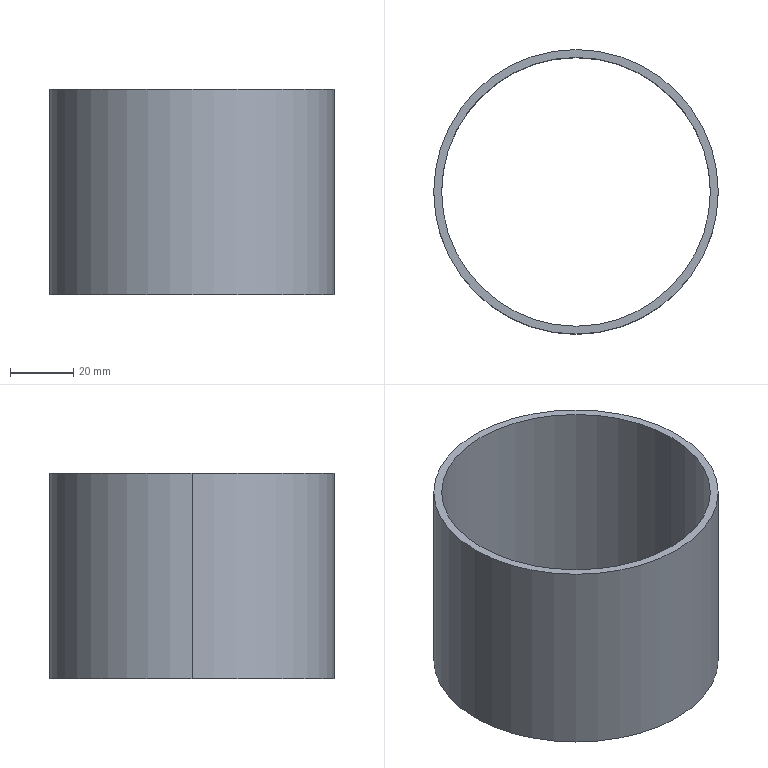Part | SolidWorks | features Extrusion 1 | 1 solid | 6 faces | box 90 x 90 x 65 mm | volume 44670 mm3 | cylinder 4 | plane 2 | commonest cylinder face diameters 85 x2 90 x2
STEP:
#1=CARTESIAN_POINT('',(-42.5,0.,32.5));
#2=VERTEX_POINT('',#1);
#3=CARTESIAN_POINT('',(42.5,0.,32.5));
#4=VERTEX_POINT('',#3);
#5=CARTESIAN_POINT('',(0.,0.,32.5));
#6=DIRECTION('',(0.,0.,1.));
#7=DIRECTION('',(1.,0.,0.));
#8=AXIS2_PLACEMENT_3D('',#5,#6,#7);
#9=CIRCLE('',#8,42.5);
#10=EDGE_CURVE('',#2,#4,#9,.T.);
#11=ORIENTED_EDGE('',*,*,#10,.T.);
#12=CARTESIAN_POINT('',(42.5,0.,-32.5));
#13=VERTEX_POINT('',#12);
#14=CARTESIAN_POINT('',(42.5,0.,32.5));
#15=DIRECTION('',(0.,0.,-1.));
#16=VECTOR('',#15,1000.);
#17=LINE('',#14,#16);
#18=EDGE_CURVE('',#4,#13,#17,.T.);
#19=ORIENTED_EDGE('',*,*,#18,.T.);
#20=CARTESIAN_POINT('',(-42.5,0.,-32.5));
#21=VERTEX_POINT('',#20);
#22=CARTESIAN_POINT('',(0.,0.,-32.5));
#23=DIRECTION('',(0.,0.,1.));
#24=DIRECTION('',(1.,0.,0.));
#25=AXIS2_PLACEMENT_3D('',#22,#23,#24);
#26=CIRCLE('',#25,42.5);
#27=EDGE_CURVE('',#21,#13,#26,.T.);
#28=ORIENTED_EDGE('',*,*,#27,.F.);
#29=CARTESIAN_POINT('',(-42.5,0.,32.5));
#30=DIRECTION('',(0.,0.,-1.));
#31=VECTOR('',#30,1000.);
#32=LINE('',#29,#31);
#33=EDGE_CURVE('',#2,#21,#32,.T.);
#34=ORIENTED_EDGE('',*,*,#33,.F.);
#35=EDGE_LOOP('',(#11,#19,#28,#34));
#36=FACE_OUTER_BOUND('',#35,.T.);
#37=CARTESIAN_POINT('',(0.,0.,32.5));
#38=DIRECTION('',(0.,0.,-1.));
#39=DIRECTION('',(-1.,0.,0.));
#40=AXIS2_PLACEMENT_3D('',#37,#38,#39);
#41=CYLINDRICAL_SURFACE('',#40,42.5);
#42=ADVANCED_FACE('',(#36),#41,.F.);
#43=CARTESIAN_POINT('',(45.,0.,32.5));
#44=VERTEX_POINT('',#43);
#45=CARTESIAN_POINT('',(-45.,0.,32.5));
#46=VERTEX_POINT('',#45);
#47=CARTESIAN_POINT('',(0.,0.,32.5));
#48=DIRECTION('',(0.,0.,1.));
#49=DIRECTION('',(1.,0.,0.));
#50=AXIS2_PLACEMENT_3D('',#47,#48,#49);
#51=CIRCLE('',#50,45.);
#52=EDGE_CURVE('',#44,#46,#51,.T.);
#53=ORIENTED_EDGE('',*,*,#52,.F.);
#54=CARTESIAN_POINT('',(45.,0.,-32.5));
#55=VERTEX_POINT('',#54);
#56=CARTESIAN_POINT('',(45.,0.,32.5));
#57=DIRECTION('',(0.,0.,-1.));
#58=VECTOR('',#57,1000.);
#59=LINE('',#56,#58);
#60=EDGE_CURVE('',#44,#55,#59,.T.);
#61=ORIENTED_EDGE('',*,*,#60,.T.);
#62=CARTESIAN_POINT('',(-45.,0.,-32.5));
#63=VERTEX_POINT('',#62);
#64=CARTESIAN_POINT('',(0.,0.,-32.5));
#65=DIRECTION('',(0.,0.,1.));
#66=DIRECTION('',(1.,0.,0.));
#67=AXIS2_PLACEMENT_3D('',#64,#65,#66);
#68=CIRCLE('',#67,45.);
#69=EDGE_CURVE('',#55,#63,#68,.T.);
#70=ORIENTED_EDGE('',*,*,#69,.T.);
#71=CARTESIAN_POINT('',(-45.,0.,32.5));
#72=DIRECTION('',(0.,0.,-1.));
#73=VECTOR('',#72,1000.);
#74=LINE('',#71,#73);
#75=EDGE_CURVE('',#46,#63,#74,.T.);
#76=ORIENTED_EDGE('',*,*,#75,.F.);
#77=EDGE_LOOP('',(#53,#61,#70,#76));
#78=FACE_OUTER_BOUND('',#77,.T.);
#79=CARTESIAN_POINT('',(0.,0.,32.5));
#80=DIRECTION('',(0.,0.,-1.));
#81=DIRECTION('',(-1.,0.,0.));
#82=AXIS2_PLACEMENT_3D('',#79,#80,#81);
#83=CYLINDRICAL_SURFACE('',#82,45.);
#84=ADVANCED_FACE('',(#78),#83,.T.);
#85=CARTESIAN_POINT('',(0.,0.,32.5));
#86=DIRECTION('',(0.,0.,1.));
#87=DIRECTION('',(1.,0.,0.));
#88=AXIS2_PLACEMENT_3D('',#85,#86,#87);
#89=CIRCLE('',#88,45.);
#90=EDGE_CURVE('',#46,#44,#89,.T.);
#91=ORIENTED_EDGE('',*,*,#90,.T.);
#92=ORIENTED_EDGE('',*,*,#52,.T.);
#93=EDGE_LOOP('',(#91,#92));
#94=FACE_OUTER_BOUND('',#93,.T.);
#95=ORIENTED_EDGE('',*,*,#10,.F.);
#96=CARTESIAN_POINT('',(0.,0.,32.5));
#97=DIRECTION('',(0.,0.,1.));
#98=DIRECTION('',(1.,0.,0.));
#99=AXIS2_PLACEMENT_3D('',#96,#97,#98);
#100=CIRCLE('',#99,42.5);
#101=EDGE_CURVE('',#4,#2,#100,.T.);
#102=ORIENTED_EDGE('',*,*,#101,.F.);
#103=EDGE_LOOP('',(#95,#102));
#104=FACE_BOUND('',#103,.T.);
#105=CARTESIAN_POINT('',(0.,0.,32.5));
#106=DIRECTION('',(0.,0.,1.));
#107=DIRECTION('',(1.,0.,0.));
#108=AXIS2_PLACEMENT_3D('',#105,#106,#107);
#109=PLANE('',#108);
#110=ADVANCED_FACE('',(#94,#104),#109,.T.);
#111=CARTESIAN_POINT('',(0.,0.,-32.5));
#112=DIRECTION('',(0.,0.,1.));
#113=DIRECTION('',(1.,0.,0.));
#114=AXIS2_PLACEMENT_3D('',#111,#112,#113);
#115=CIRCLE('',#114,45.);
#116=EDGE_CURVE('',#63,#55,#115,.T.);
#117=ORIENTED_EDGE('',*,*,#116,.F.);
#118=ORIENTED_EDGE('',*,*,#69,.F.);
#119=EDGE_LOOP('',(#117,#118));
#120=FACE_OUTER_BOUND('',#119,.T.);
#121=ORIENTED_EDGE('',*,*,#27,.T.);
#122=CARTESIAN_POINT('',(0.,0.,-32.5));
#123=DIRECTION('',(0.,0.,1.));
#124=DIRECTION('',(1.,0.,0.));
#125=AXIS2_PLACEMENT_3D('',#122,#123,#124);
#126=CIRCLE('',#125,42.5);
#127=EDGE_CURVE('',#13,#21,#126,.T.);
#128=ORIENTED_EDGE('',*,*,#127,.T.);
#129=EDGE_LOOP('',(#121,#128));
#130=FACE_BOUND('',#129,.T.);
#131=CARTESIAN_POINT('',(0.,0.,-32.5));
#132=DIRECTION('',(0.,0.,1.));
#133=DIRECTION('',(1.,0.,0.));
#134=AXIS2_PLACEMENT_3D('',#131,#132,#133);
#135=PLANE('',#134);
#136=ADVANCED_FACE('',(#120,#130),#135,.F.);
#137=ORIENTED_EDGE('',*,*,#60,.F.);
#138=ORIENTED_EDGE('',*,*,#90,.F.);
#139=ORIENTED_EDGE('',*,*,#75,.T.);
#140=ORIENTED_EDGE('',*,*,#116,.T.);
#141=EDGE_LOOP('',(#137,#138,#139,#140));
#142=FACE_OUTER_BOUND('',#141,.T.);
#143=CARTESIAN_POINT('',(0.,0.,32.5));
#144=DIRECTION('',(0.,0.,-1.));
#145=DIRECTION('',(-1.,0.,0.));
#146=AXIS2_PLACEMENT_3D('',#143,#144,#145);
#147=CYLINDRICAL_SURFACE('',#146,45.);
#148=ADVANCED_FACE('',(#142),#147,.T.);
#149=ORIENTED_EDGE('',*,*,#18,.F.);
#150=ORIENTED_EDGE('',*,*,#101,.T.);
#151=ORIENTED_EDGE('',*,*,#33,.T.);
#152=ORIENTED_EDGE('',*,*,#127,.F.);
#153=EDGE_LOOP('',(#149,#150,#151,#152));
#154=FACE_OUTER_BOUND('',#153,.T.);
#155=CARTESIAN_POINT('',(0.,0.,32.5));
#156=DIRECTION('',(0.,0.,-1.));
#157=DIRECTION('',(-1.,0.,0.));
#158=AXIS2_PLACEMENT_3D('',#155,#156,#157);
#159=CYLINDRICAL_SURFACE('',#158,42.5);
#160=ADVANCED_FACE('',(#154),#159,.F.);
#161=CLOSED_SHELL('',(#42,#84,#110,#136,#148,#160));
#162=MANIFOLD_SOLID_BREP('',#161);
#163=CARTESIAN_POINT('',(0.,0.,0.));
#164=DIRECTION('',(0.,0.,1.));
#165=DIRECTION('',(1.,0.,0.));
#166=AXIS2_PLACEMENT_3D('',#163,#164,#165);
#167=(LENGTH_UNIT()NAMED_UNIT(*)SI_UNIT(.MILLI.,.METRE.));
#168=UNCERTAINTY_MEASURE_WITH_UNIT(LENGTH_MEASURE(0.00001),#167,'','');
#169=(NAMED_UNIT(*)PLANE_ANGLE_UNIT()SI_UNIT($,.RADIAN.));
#170=(NAMED_UNIT(*)SI_UNIT($,.STERADIAN.)SOLID_ANGLE_UNIT());
#171=(GEOMETRIC_REPRESENTATION_CONTEXT(3)GLOBAL_UNCERTAINTY_ASSIGNED_CONTEXT((#168))GLOBAL_UNIT_ASSIGNED_CONTEXT((#167,#169,#170))REPRESENTATION_CONTEXT('',''));
#172=ADVANCED_BREP_SHAPE_REPRESENTATION('',(#162,#166),#171);